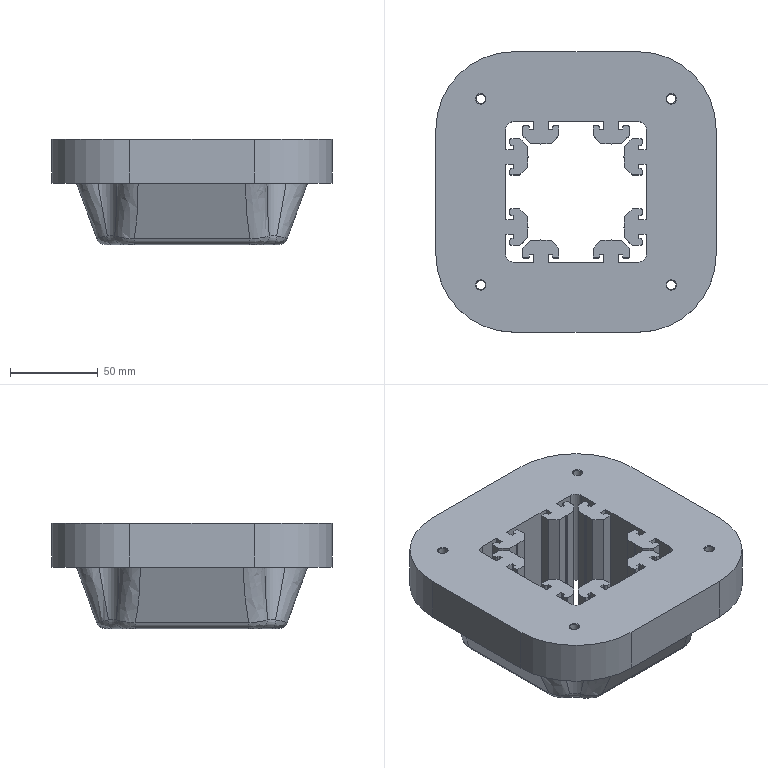Part | NX | features BREP 1 | 1 solid | 239 faces | box 159.676 x 159.676 x 60 mm | volume 741091 mm3 | plane 155 | cylinder 56 | spline 16 | cone 8 | torus 4 | commonest cylinder face diameters 1 x16 2 x16 5.2 x4 9 x4 10 x4 16 x4